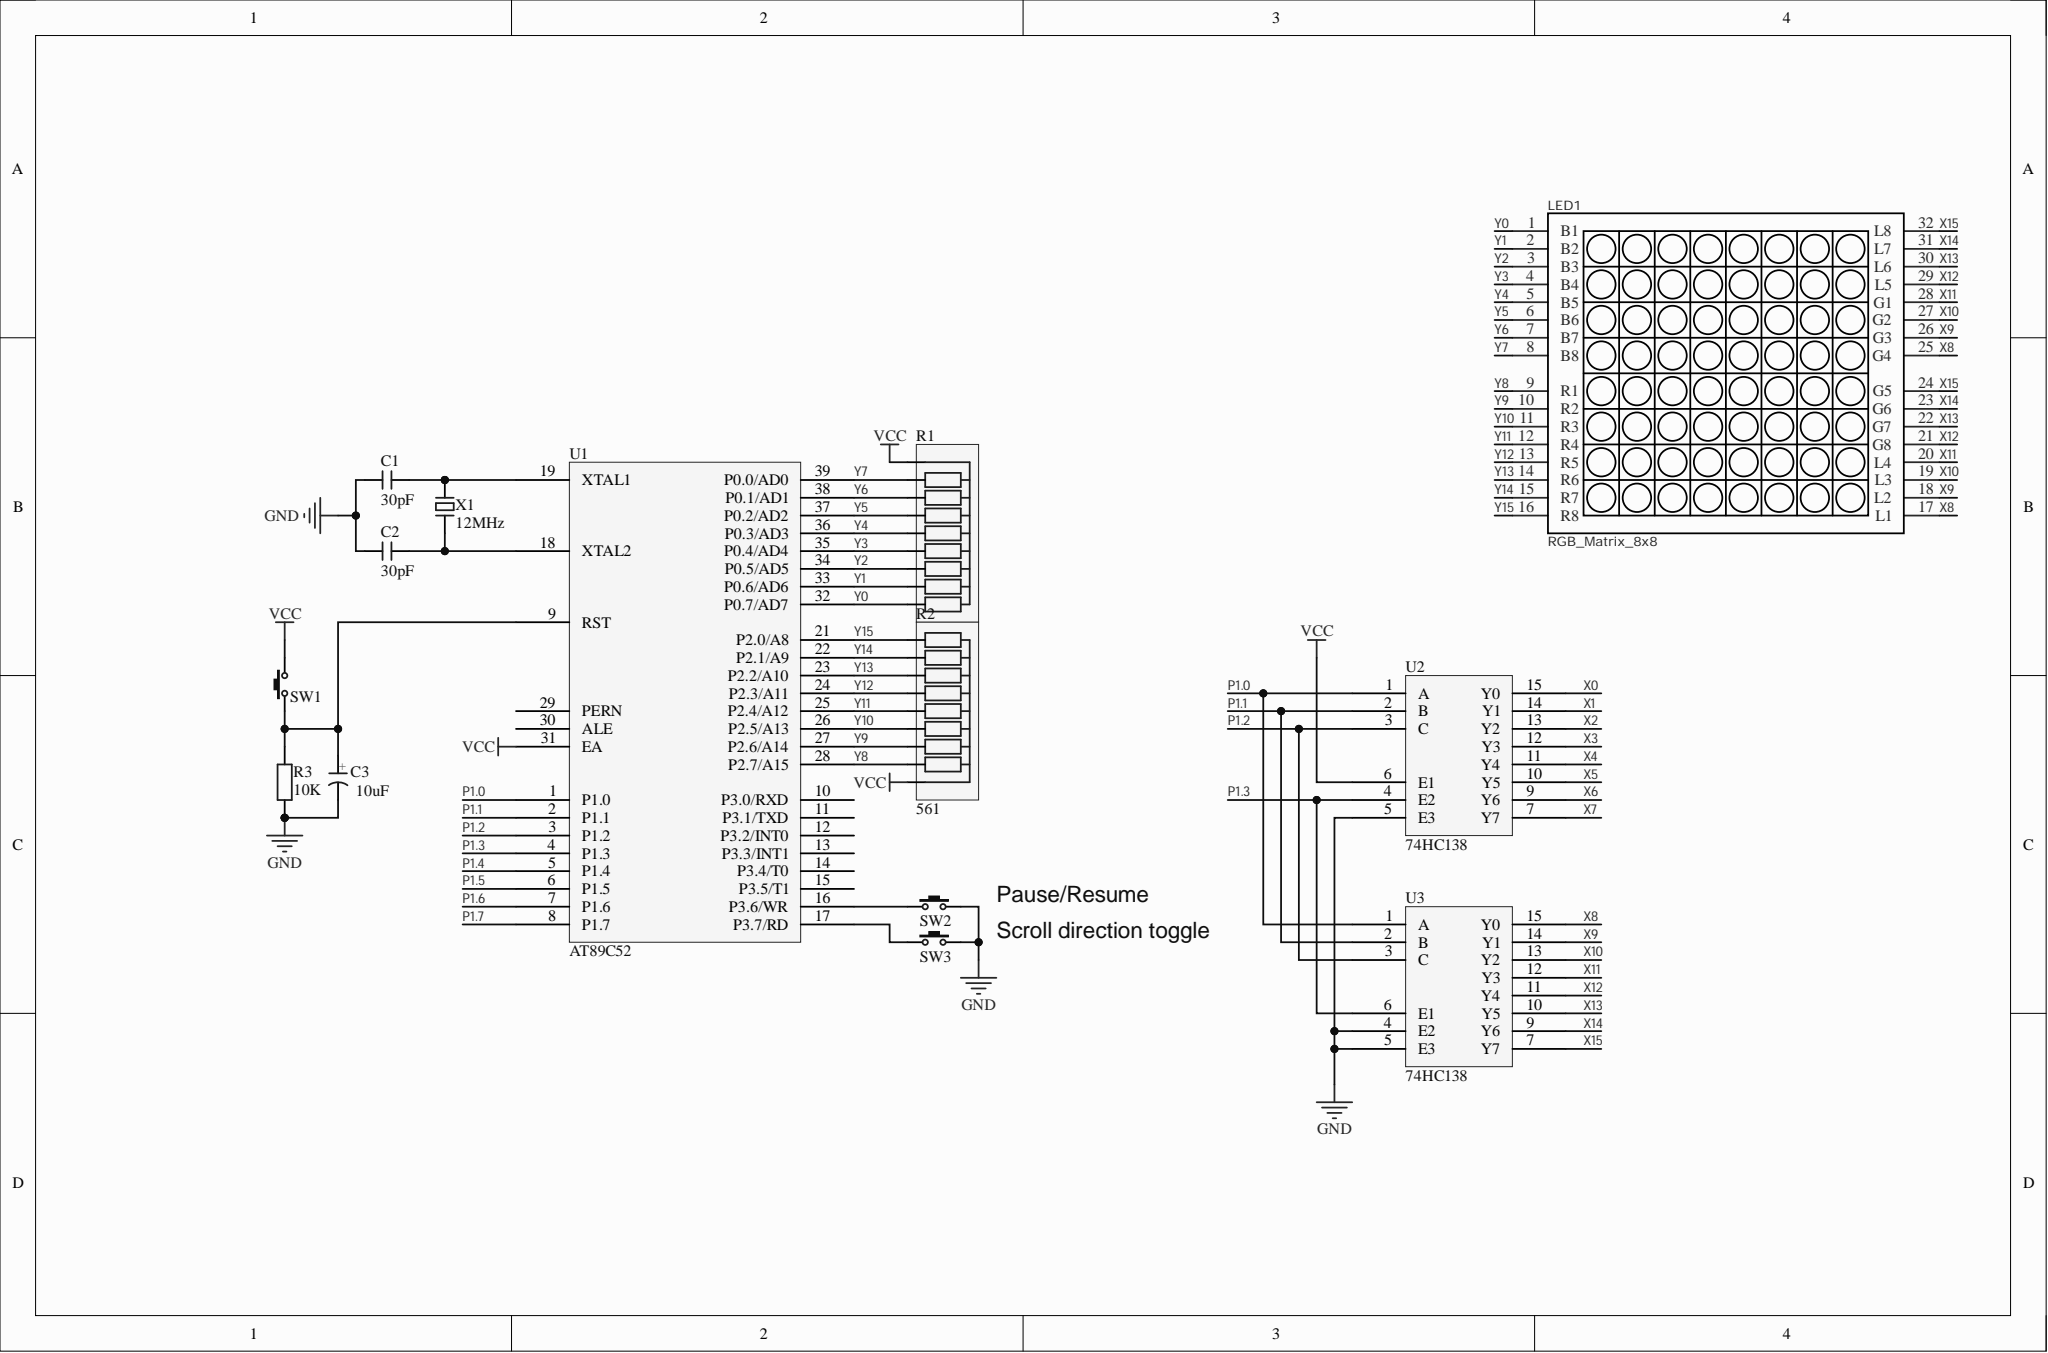Circuit board | Altium Designer | 14 parts | 35 nets
Bill of materials:
Comment,Description,Designator,Footprint,LibRef,Quantity
"30pF","Non-polar SMD capacitor","C1, C2","CC 1.8*3.6","C","2"
"10uF","THT electrolytic capacitor","C3","CAP 1.5*4*8","C-CAP","1"
"RGB_Matrix_8x8","","LED1","RGB_MATRIX_8X8","RGB_Matrix_8x8","1"
"561","Single in-line resistor array","R1, R2","R SIP9-2.54","R SIP9","2"
"10K","SMD resistor","R3","RS 1/8W","R","1"
"3x6x5","3x6 tact switch","SW1, SW2, SW3","TSW DIP-3*6*5","TSW 3x6","3"
"AT89C52","","U1","DIP40","AT89C52","1"
"74HC138","","U2, U3","648-08","Component_1","2"
"12MHz","2-pin passive crystal","X1","OSC HC-49S","XTAL-2P","1"
Netlist (Protel format):
[
C1
CC 1.8*3.6
30pF



]
[
C2
CC 1.8*3.6
30pF



]
[
C3
CAP 1.5*4*8
10uF



]
[
LED1
RGB_MATRIX_8X8
RGB_Matrix_8x8



]
[
R1
R SIP9-2.54
561



]
[
R2
R SIP9-2.54
561



]
[
R3
RS 1/8W
10K



]
[
SW1
TSW DIP-3*6*5
3x6x5



]
[
SW2
TSW DIP-3*6*5
3x6x5



]
[
SW3
TSW DIP-3*6*5
3x6x5



]
[
U1
DIP40
AT89C52



]
[
U2
648-08
74HC138



]
[
U3
648-08
74HC138



]
[
X1
OSC HC-49S
12MHz



]
(
Y15
LED1-16
R2-9
U1-21
)
(
Y14
LED1-15
R2-8
U1-22
)
(
Y13
LED1-14
R2-7
U1-23
)
(
Y12
LED1-13
R2-6
U1-24
)
(
Y11
LED1-12
R2-5
U1-25
)
(
Y10
LED1-11
R2-4
U1-26
)
(
Y9
LED1-10
R2-3
U1-27
)
(
Y8
LED1-9
R2-2
U1-28
)
(
Y7
LED1-8
R1-2
U1-39
)
(
Y6
LED1-7
R1-3
U1-38
)
(
Y5
LED1-6
R1-4
U1-37
)
(
Y4
LED1-5
R1-5
U1-36
)
(
Y3
LED1-4
R1-6
U1-35
)
(
Y2
LED1-3
R1-7
U1-34
)
(
Y1
LED1-2
R1-8
U1-33
)
(
Y0
LED1-1
R1-9
U1-32
)
(
X15
LED1-24
LED1-32
U3-7
)
(
X14
LED1-23
LED1-31
U3-9
)
(
X13
LED1-22
LED1-30
U3-10
)
(
X12
LED1-21
LED1-29
U3-11
)
(
X11
LED1-20
LED1-28
U3-12
)
(
X10
LED1-19
LED1-27
U3-13
)
(
X9
LED1-18
LED1-26
U3-14
)
(
X8
LED1-17
LED1-25
U3-15
)
(
VCC
R1-1
R2-1
SW1-2
U1-31
U2-6
)
(
P1.3
U1-4
U2-4
U3-6
)
(
P1.2
U1-3
U2-3
U3-3
)
(
P1.1
U1-2
U2-2
U3-2
)
(
P1.0
U1-1
U2-1
U3-1
)
(
NetSW3_1
SW3-1
U1-17
)
(
NetSW2_1
SW2-1
U1-16
)
(
NetC3_1
C3-1
R3-2
SW1-1
U1-9
)
(
NetC2_2
C2-2
U1-18
X1-1
)
(
NetC1_2
C1-2
U1-19
X1-2
)
(
GND
C1-1
C2-1
C3-2
R3-1
SW2-2
SW3-2
U2-5
U3-4
U3-5
)